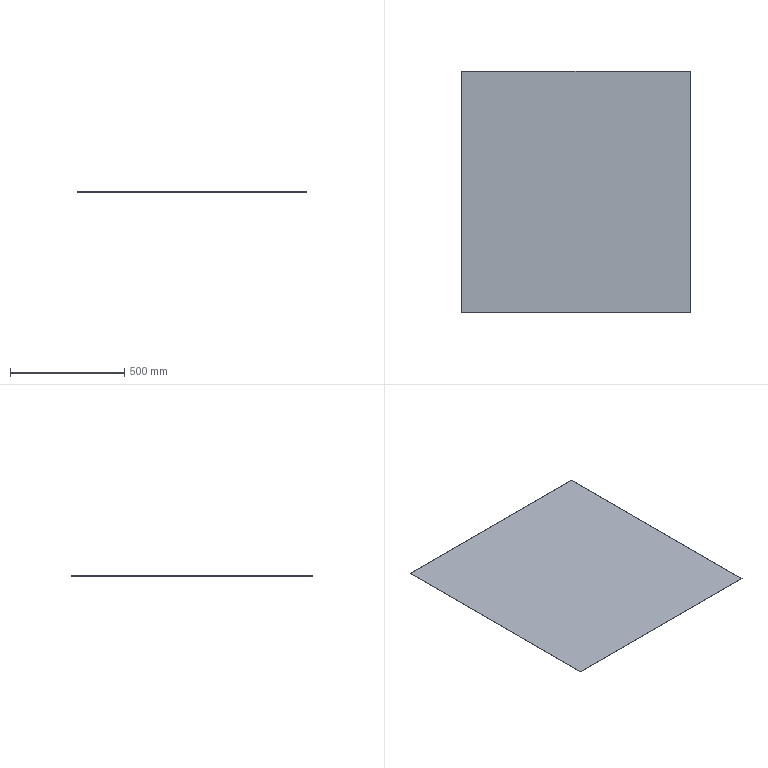Part | SolidWorks | features FlatPattern 1, SMBaseFlange 1, SheetMetal 1 | 1 solid | 6 faces | box 998.4 x 1055 x 0.8 mm | volume 842809 mm3 | plane 6
STEP:
#1=CARTESIAN_POINT('',(-18.276,41.031,0.));
#2=VERTEX_POINT('',#1);
#3=CARTESIAN_POINT('',(21.031,41.031,0.));
#4=VERTEX_POINT('',#3);
#5=CARTESIAN_POINT('',(-18.276,41.031,0.));
#6=DIRECTION('',(1.,0.,0.));
#7=VECTOR('',#6,39.37);
#8=LINE('',#5,#7);
#9=EDGE_CURVE('',#2,#4,#8,.T.);
#10=ORIENTED_EDGE('',*,*,#9,.F.);
#11=CARTESIAN_POINT('',(-18.276,41.031,0.0315));
#12=VERTEX_POINT('',#11);
#13=CARTESIAN_POINT('',(-18.276,41.031,0.0315));
#14=DIRECTION('',(0.,0.,-1.));
#15=VECTOR('',#14,39.37);
#16=LINE('',#13,#15);
#17=EDGE_CURVE('',#12,#2,#16,.T.);
#18=ORIENTED_EDGE('',*,*,#17,.F.);
#19=CARTESIAN_POINT('',(21.031,41.031,0.0315));
#20=VERTEX_POINT('',#19);
#21=CARTESIAN_POINT('',(-18.276,41.031,0.0315));
#22=DIRECTION('',(1.,0.,0.));
#23=VECTOR('',#22,39.37);
#24=LINE('',#21,#23);
#25=EDGE_CURVE('',#12,#20,#24,.T.);
#26=ORIENTED_EDGE('',*,*,#25,.T.);
#27=CARTESIAN_POINT('',(21.031,41.031,0.0315));
#28=DIRECTION('',(0.,0.,-1.));
#29=VECTOR('',#28,39.37);
#30=LINE('',#27,#29);
#31=EDGE_CURVE('',#20,#4,#30,.T.);
#32=ORIENTED_EDGE('',*,*,#31,.T.);
#33=EDGE_LOOP('',(#10,#18,#26,#32));
#34=FACE_OUTER_BOUND('',#33,.T.);
#35=CARTESIAN_POINT('',(-18.276,41.031,0.0315));
#36=DIRECTION('',(0.,1.,0.));
#37=DIRECTION('',(0.,0.,1.));
#38=AXIS2_PLACEMENT_3D('',#35,#36,#37);
#39=PLANE('',#38);
#40=ADVANCED_FACE('',(#34),#39,.T.);
#41=CARTESIAN_POINT('',(-18.276,-0.5118,0.));
#42=VERTEX_POINT('',#41);
#43=CARTESIAN_POINT('',(-18.276,-0.5118,0.));
#44=DIRECTION('',(0.,1.,0.));
#45=VECTOR('',#44,39.37);
#46=LINE('',#43,#45);
#47=EDGE_CURVE('',#42,#2,#46,.T.);
#48=ORIENTED_EDGE('',*,*,#47,.F.);
#49=CARTESIAN_POINT('',(-18.276,-0.5118,0.0315));
#50=VERTEX_POINT('',#49);
#51=CARTESIAN_POINT('',(-18.276,-0.5118,0.0315));
#52=DIRECTION('',(0.,0.,-1.));
#53=VECTOR('',#52,39.37);
#54=LINE('',#51,#53);
#55=EDGE_CURVE('',#50,#42,#54,.T.);
#56=ORIENTED_EDGE('',*,*,#55,.F.);
#57=CARTESIAN_POINT('',(-18.276,-0.5118,0.0315));
#58=DIRECTION('',(0.,1.,0.));
#59=VECTOR('',#58,39.37);
#60=LINE('',#57,#59);
#61=EDGE_CURVE('',#50,#12,#60,.T.);
#62=ORIENTED_EDGE('',*,*,#61,.T.);
#63=ORIENTED_EDGE('',*,*,#17,.T.);
#64=EDGE_LOOP('',(#48,#56,#62,#63));
#65=FACE_OUTER_BOUND('',#64,.T.);
#66=CARTESIAN_POINT('',(-18.276,-0.5118,0.0315));
#67=DIRECTION('',(-1.,0.,0.));
#68=DIRECTION('',(0.,0.,1.));
#69=AXIS2_PLACEMENT_3D('',#66,#67,#68);
#70=PLANE('',#69);
#71=ADVANCED_FACE('',(#65),#70,.T.);
#72=CARTESIAN_POINT('',(21.031,-0.5118,0.));
#73=VERTEX_POINT('',#72);
#74=CARTESIAN_POINT('',(21.031,-0.5118,0.));
#75=DIRECTION('',(-1.,0.,0.));
#76=VECTOR('',#75,39.37);
#77=LINE('',#74,#76);
#78=EDGE_CURVE('',#73,#42,#77,.T.);
#79=ORIENTED_EDGE('',*,*,#78,.F.);
#80=CARTESIAN_POINT('',(21.031,-0.5118,0.0315));
#81=VERTEX_POINT('',#80);
#82=CARTESIAN_POINT('',(21.031,-0.5118,0.0315));
#83=DIRECTION('',(0.,0.,-1.));
#84=VECTOR('',#83,39.37);
#85=LINE('',#82,#84);
#86=EDGE_CURVE('',#81,#73,#85,.T.);
#87=ORIENTED_EDGE('',*,*,#86,.F.);
#88=CARTESIAN_POINT('',(21.031,-0.5118,0.0315));
#89=DIRECTION('',(-1.,0.,0.));
#90=VECTOR('',#89,39.37);
#91=LINE('',#88,#90);
#92=EDGE_CURVE('',#81,#50,#91,.T.);
#93=ORIENTED_EDGE('',*,*,#92,.T.);
#94=ORIENTED_EDGE('',*,*,#55,.T.);
#95=EDGE_LOOP('',(#79,#87,#93,#94));
#96=FACE_OUTER_BOUND('',#95,.T.);
#97=CARTESIAN_POINT('',(21.031,-0.5118,0.0315));
#98=DIRECTION('',(0.,-1.,0.));
#99=DIRECTION('',(0.,0.,-1.));
#100=AXIS2_PLACEMENT_3D('',#97,#98,#99);
#101=PLANE('',#100);
#102=ADVANCED_FACE('',(#96),#101,.T.);
#103=CARTESIAN_POINT('',(21.031,41.031,0.));
#104=DIRECTION('',(0.,-1.,0.));
#105=VECTOR('',#104,39.37);
#106=LINE('',#103,#105);
#107=EDGE_CURVE('',#4,#73,#106,.T.);
#108=ORIENTED_EDGE('',*,*,#107,.F.);
#109=ORIENTED_EDGE('',*,*,#31,.F.);
#110=CARTESIAN_POINT('',(21.031,41.031,0.0315));
#111=DIRECTION('',(0.,-1.,0.));
#112=VECTOR('',#111,39.37);
#113=LINE('',#110,#112);
#114=EDGE_CURVE('',#20,#81,#113,.T.);
#115=ORIENTED_EDGE('',*,*,#114,.T.);
#116=ORIENTED_EDGE('',*,*,#86,.T.);
#117=EDGE_LOOP('',(#108,#109,#115,#116));
#118=FACE_OUTER_BOUND('',#117,.T.);
#119=CARTESIAN_POINT('',(21.031,41.031,0.0315));
#120=DIRECTION('',(1.,0.,0.));
#121=DIRECTION('',(0.,1.,0.));
#122=AXIS2_PLACEMENT_3D('',#119,#120,#121);
#123=PLANE('',#122);
#124=ADVANCED_FACE('',(#118),#123,.T.);
#125=ORIENTED_EDGE('',*,*,#25,.F.);
#126=ORIENTED_EDGE('',*,*,#61,.F.);
#127=ORIENTED_EDGE('',*,*,#92,.F.);
#128=ORIENTED_EDGE('',*,*,#114,.F.);
#129=EDGE_LOOP('',(#125,#126,#127,#128));
#130=FACE_OUTER_BOUND('',#129,.T.);
#131=CARTESIAN_POINT('',(0.,0.,0.0315));
#132=DIRECTION('',(0.,0.,-1.));
#133=DIRECTION('',(0.,1.,0.));
#134=AXIS2_PLACEMENT_3D('',#131,#132,#133);
#135=PLANE('',#134);
#136=ADVANCED_FACE('',(#130),#135,.F.);
#137=ORIENTED_EDGE('',*,*,#9,.T.);
#138=ORIENTED_EDGE('',*,*,#107,.T.);
#139=ORIENTED_EDGE('',*,*,#78,.T.);
#140=ORIENTED_EDGE('',*,*,#47,.T.);
#141=EDGE_LOOP('',(#137,#138,#139,#140));
#142=FACE_OUTER_BOUND('',#141,.T.);
#143=CARTESIAN_POINT('',(0.,0.,0.));
#144=DIRECTION('',(0.,0.,-1.));
#145=DIRECTION('',(0.,1.,0.));
#146=AXIS2_PLACEMENT_3D('',#143,#144,#145);
#147=PLANE('',#146);
#148=ADVANCED_FACE('',(#142),#147,.T.);
#149=CLOSED_SHELL('',(#40,#71,#102,#124,#136,#148));
#150=MANIFOLD_SOLID_BREP('',#149);
#151=CARTESIAN_POINT('',(0.,0.,0.));
#152=DIRECTION('',(0.,0.,1.));
#153=DIRECTION('',(1.,0.,0.));
#154=AXIS2_PLACEMENT_3D('',#151,#152,#153);
#155=(LENGTH_UNIT()NAMED_UNIT(*)SI_UNIT($,.METRE.));
#156=LENGTH_MEASURE_WITH_UNIT(LENGTH_MEASURE(0.0254),#155);
#157=DIMENSIONAL_EXPONENTS(1.,0.,0.,0.,0.,0.,0.);
#158=(CONVERSION_BASED_UNIT('INCH',#156)LENGTH_UNIT()NAMED_UNIT(#157));
#159=UNCERTAINTY_MEASURE_WITH_UNIT(LENGTH_MEASURE(0.00001),#158,'','');
#160=(NAMED_UNIT(*)PLANE_ANGLE_UNIT()SI_UNIT($,.RADIAN.));
#161=(NAMED_UNIT(*)SI_UNIT($,.STERADIAN.)SOLID_ANGLE_UNIT());
#162=(GEOMETRIC_REPRESENTATION_CONTEXT(3)GLOBAL_UNCERTAINTY_ASSIGNED_CONTEXT((#159))GLOBAL_UNIT_ASSIGNED_CONTEXT((#158,#160,#161))REPRESENTATION_CONTEXT('',''));
#163=ADVANCED_BREP_SHAPE_REPRESENTATION('',(#150,#154),#162);